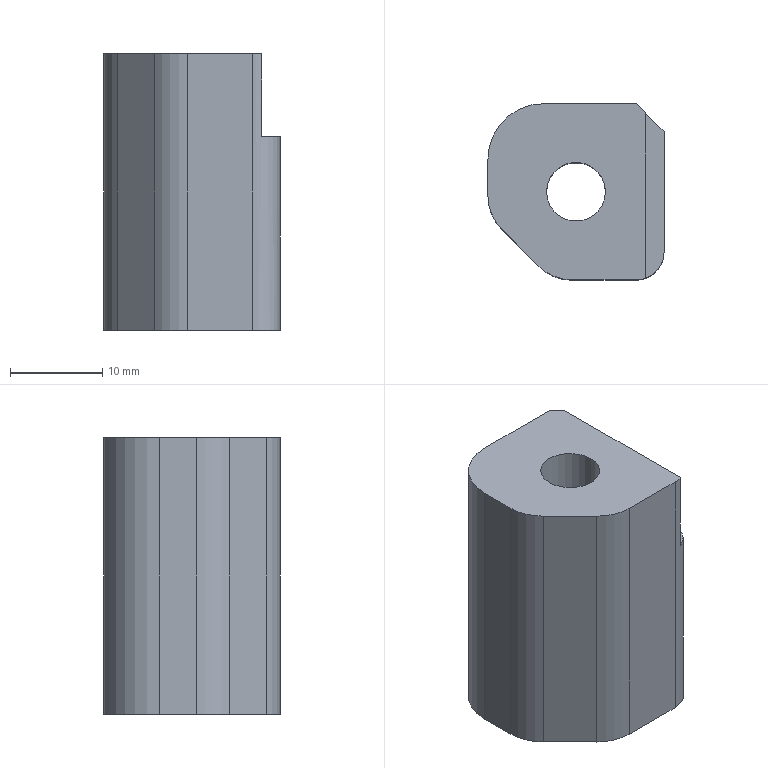Part | STEP file | 1 solid | 15 faces | box 19.1 x 19.1 x 30 mm | volume 8502 mm3 | plane 10 | cylinder 5 | commonest cylinder face diameters 10 x2 6 x1 6.38 x1 12 x1
STEP:
#1=CARTESIAN_POINT('',(-238.45,-56.55,-2.));
#2=VERTEX_POINT('',#1);
#3=CARTESIAN_POINT('',(-245.479,-56.55,-2.));
#4=VERTEX_POINT('',#3);
#5=CARTESIAN_POINT('',(-245.,-56.55,-2.));
#6=DIRECTION('',(-1.,0.,0.));
#7=VECTOR('',#6,1.);
#8=LINE('',#5,#7);
#9=EDGE_CURVE('',#2,#4,#8,.T.);
#10=ORIENTED_EDGE('',*,*,#9,.T.);
#11=CARTESIAN_POINT('',(-245.479,-56.55,-32.));
#12=VERTEX_POINT('',#11);
#13=CARTESIAN_POINT('',(-245.479,-56.55,-30.));
#14=DIRECTION('',(0.,0.,-1.));
#15=VECTOR('',#14,1.);
#16=LINE('',#13,#15);
#17=EDGE_CURVE('',#4,#12,#16,.T.);
#18=ORIENTED_EDGE('',*,*,#17,.T.);
#19=CARTESIAN_POINT('',(-238.45,-56.55,-32.));
#20=VERTEX_POINT('',#19);
#21=CARTESIAN_POINT('',(-245.,-56.55,-32.));
#22=DIRECTION('',(1.,0.,0.));
#23=VECTOR('',#22,1.);
#24=LINE('',#21,#23);
#25=EDGE_CURVE('',#12,#20,#24,.T.);
#26=ORIENTED_EDGE('',*,*,#25,.T.);
#27=CARTESIAN_POINT('',(-238.45,-56.55,-30.));
#28=DIRECTION('',(0.,0.,1.));
#29=VECTOR('',#28,1.);
#30=LINE('',#27,#29);
#31=EDGE_CURVE('',#20,#2,#30,.T.);
#32=ORIENTED_EDGE('',*,*,#31,.T.);
#33=EDGE_LOOP('',(#10,#18,#26,#32));
#34=FACE_OUTER_BOUND('',#33,.T.);
#35=CARTESIAN_POINT('',(-245.,-56.55,-30.));
#36=DIRECTION('',(0.,-1.,0.));
#37=DIRECTION('',(0.,0.,-1.));
#38=AXIS2_PLACEMENT_3D('',#35,#36,#37);
#39=PLANE('',#38);
#40=ADVANCED_FACE('',(#34),#39,.T.);
#41=CARTESIAN_POINT('',(-254.55,-43.45,-32.));
#42=VERTEX_POINT('',#41);
#43=CARTESIAN_POINT('',(-254.55,-47.479,-32.));
#44=VERTEX_POINT('',#43);
#45=CARTESIAN_POINT('',(-254.55,-47.,-32.));
#46=DIRECTION('',(0.,-1.,0.));
#47=VECTOR('',#46,1.);
#48=LINE('',#45,#47);
#49=EDGE_CURVE('',#42,#44,#48,.T.);
#50=ORIENTED_EDGE('',*,*,#49,.T.);
#51=CARTESIAN_POINT('',(-254.55,-47.479,-2.));
#52=VERTEX_POINT('',#51);
#53=CARTESIAN_POINT('',(-254.55,-47.479,-30.));
#54=DIRECTION('',(0.,0.,1.));
#55=VECTOR('',#54,1.);
#56=LINE('',#53,#55);
#57=EDGE_CURVE('',#44,#52,#56,.T.);
#58=ORIENTED_EDGE('',*,*,#57,.T.);
#59=CARTESIAN_POINT('',(-254.55,-43.45,-2.));
#60=VERTEX_POINT('',#59);
#61=CARTESIAN_POINT('',(-254.55,-47.,-2.));
#62=DIRECTION('',(0.,1.,0.));
#63=VECTOR('',#62,1.);
#64=LINE('',#61,#63);
#65=EDGE_CURVE('',#52,#60,#64,.T.);
#66=ORIENTED_EDGE('',*,*,#65,.T.);
#67=CARTESIAN_POINT('',(-254.55,-43.45,-30.));
#68=DIRECTION('',(0.,0.,-1.));
#69=VECTOR('',#68,1.);
#70=LINE('',#67,#69);
#71=EDGE_CURVE('',#60,#42,#70,.T.);
#72=ORIENTED_EDGE('',*,*,#71,.T.);
#73=EDGE_LOOP('',(#50,#58,#66,#72));
#74=FACE_OUTER_BOUND('',#73,.T.);
#75=CARTESIAN_POINT('',(-254.55,-47.,-30.));
#76=DIRECTION('',(-1.,0.,0.));
#77=DIRECTION('',(0.,0.,1.));
#78=AXIS2_PLACEMENT_3D('',#75,#76,#77);
#79=PLANE('',#78);
#80=ADVANCED_FACE('',(#74),#79,.T.);
#81=CARTESIAN_POINT('',(-248.55,-37.45,-32.));
#82=VERTEX_POINT('',#81);
#83=CARTESIAN_POINT('',(-248.55,-37.45,-2.));
#84=VERTEX_POINT('',#83);
#85=CARTESIAN_POINT('',(-248.55,-37.45,-30.));
#86=DIRECTION('',(0.,0.,1.));
#87=VECTOR('',#86,1.);
#88=LINE('',#85,#87);
#89=EDGE_CURVE('',#82,#84,#88,.T.);
#90=ORIENTED_EDGE('',*,*,#89,.T.);
#91=CARTESIAN_POINT('',(-238.45,-37.45,-2.));
#92=VERTEX_POINT('',#91);
#93=CARTESIAN_POINT('',(-245.,-37.45,-2.));
#94=DIRECTION('',(1.,0.,0.));
#95=VECTOR('',#94,1.);
#96=LINE('',#93,#95);
#97=EDGE_CURVE('',#84,#92,#96,.T.);
#98=ORIENTED_EDGE('',*,*,#97,.T.);
#99=CARTESIAN_POINT('',(-238.45,-37.45,-32.));
#100=VERTEX_POINT('',#99);
#101=CARTESIAN_POINT('',(-238.45,-37.45,-30.));
#102=DIRECTION('',(0.,0.,-1.));
#103=VECTOR('',#102,1.);
#104=LINE('',#101,#103);
#105=EDGE_CURVE('',#92,#100,#104,.T.);
#106=ORIENTED_EDGE('',*,*,#105,.T.);
#107=CARTESIAN_POINT('',(-245.,-37.45,-32.));
#108=DIRECTION('',(-1.,0.,0.));
#109=VECTOR('',#108,1.);
#110=LINE('',#107,#109);
#111=EDGE_CURVE('',#100,#82,#110,.T.);
#112=ORIENTED_EDGE('',*,*,#111,.T.);
#113=EDGE_LOOP('',(#90,#98,#106,#112));
#114=FACE_OUTER_BOUND('',#113,.T.);
#115=CARTESIAN_POINT('',(-245.,-37.45,-30.));
#116=DIRECTION('',(0.,1.,0.));
#117=DIRECTION('',(0.,0.,1.));
#118=AXIS2_PLACEMENT_3D('',#115,#116,#117);
#119=PLANE('',#118);
#120=ADVANCED_FACE('',(#114),#119,.T.);
#121=CARTESIAN_POINT('',(-248.19,-47.,-32.));
#122=VERTEX_POINT('',#121);
#123=CARTESIAN_POINT('',(-245.,-47.,-32.));
#124=DIRECTION('',(0.,0.,1.));
#125=DIRECTION('',(-1.,0.,0.));
#126=AXIS2_PLACEMENT_3D('',#123,#124,#125);
#127=CIRCLE('',#126,3.19);
#128=EDGE_CURVE('',#122,#122,#127,.T.);
#129=ORIENTED_EDGE('',*,*,#128,.T.);
#130=EDGE_LOOP('',(#129));
#131=FACE_BOUND('',#130,.T.);
#132=ORIENTED_EDGE('',*,*,#25,.F.);
#133=CARTESIAN_POINT('',(-249.014,-55.086,-32.));
#134=VERTEX_POINT('',#133);
#135=CARTESIAN_POINT('',(-245.479,-51.55,-32.));
#136=DIRECTION('',(0.,0.,-1.));
#137=DIRECTION('',(-1.,0.,0.));
#138=AXIS2_PLACEMENT_3D('',#135,#136,#137);
#139=CIRCLE('',#138,5.);
#140=EDGE_CURVE('',#12,#134,#139,.T.);
#141=ORIENTED_EDGE('',*,*,#140,.T.);
#142=CARTESIAN_POINT('',(-253.086,-51.014,-32.));
#143=VERTEX_POINT('',#142);
#144=CARTESIAN_POINT('',(-251.05,-53.05,-32.));
#145=DIRECTION('',(-0.7071,0.7071,0.));
#146=VECTOR('',#145,1.);
#147=LINE('',#144,#146);
#148=EDGE_CURVE('',#134,#143,#147,.T.);
#149=ORIENTED_EDGE('',*,*,#148,.T.);
#150=CARTESIAN_POINT('',(-249.55,-47.479,-32.));
#151=DIRECTION('',(0.,0.,-1.));
#152=DIRECTION('',(-1.,0.,0.));
#153=AXIS2_PLACEMENT_3D('',#150,#151,#152);
#154=CIRCLE('',#153,5.);
#155=EDGE_CURVE('',#143,#44,#154,.T.);
#156=ORIENTED_EDGE('',*,*,#155,.T.);
#157=ORIENTED_EDGE('',*,*,#49,.F.);
#158=CARTESIAN_POINT('',(-248.55,-43.45,-32.));
#159=DIRECTION('',(0.,0.,-1.));
#160=DIRECTION('',(-1.,0.,0.));
#161=AXIS2_PLACEMENT_3D('',#158,#159,#160);
#162=CIRCLE('',#161,6.);
#163=EDGE_CURVE('',#42,#82,#162,.T.);
#164=ORIENTED_EDGE('',*,*,#163,.T.);
#165=ORIENTED_EDGE('',*,*,#111,.F.);
#166=CARTESIAN_POINT('',(-235.45,-40.45,-32.));
#167=VERTEX_POINT('',#166);
#168=CARTESIAN_POINT('',(-236.95,-38.95,-32.));
#169=DIRECTION('',(0.7071,-0.7071,0.));
#170=VECTOR('',#169,1.);
#171=LINE('',#168,#170);
#172=EDGE_CURVE('',#100,#167,#171,.T.);
#173=ORIENTED_EDGE('',*,*,#172,.T.);
#174=CARTESIAN_POINT('',(-235.45,-53.55,-32.));
#175=VERTEX_POINT('',#174);
#176=CARTESIAN_POINT('',(-235.45,-47.,-32.));
#177=DIRECTION('',(0.,1.,0.));
#178=VECTOR('',#177,1.);
#179=LINE('',#176,#178);
#180=EDGE_CURVE('',#175,#167,#179,.T.);
#181=ORIENTED_EDGE('',*,*,#180,.F.);
#182=CARTESIAN_POINT('',(-238.45,-53.55,-32.));
#183=DIRECTION('',(0.,0.,-1.));
#184=DIRECTION('',(-1.,0.,0.));
#185=AXIS2_PLACEMENT_3D('',#182,#183,#184);
#186=CIRCLE('',#185,3.);
#187=EDGE_CURVE('',#175,#20,#186,.T.);
#188=ORIENTED_EDGE('',*,*,#187,.T.);
#189=EDGE_LOOP('',(#132,#141,#149,#156,#157,#164,#165,#173,#181,#188));
#190=FACE_BOUND('',#189,.T.);
#191=CARTESIAN_POINT('',(-245.,-47.,-32.));
#192=DIRECTION('',(0.,0.,-1.));
#193=DIRECTION('',(-1.,0.,0.));
#194=AXIS2_PLACEMENT_3D('',#191,#192,#193);
#195=PLANE('',#194);
#196=ADVANCED_FACE('',(#131,#190),#195,.T.);
#197=CARTESIAN_POINT('',(-235.45,-40.45,-11.));
#198=VERTEX_POINT('',#197);
#199=CARTESIAN_POINT('',(-235.45,-53.55,-11.));
#200=VERTEX_POINT('',#199);
#201=CARTESIAN_POINT('',(-235.45,-47.,-11.));
#202=DIRECTION('',(0.,-1.,0.));
#203=VECTOR('',#202,1.);
#204=LINE('',#201,#203);
#205=EDGE_CURVE('',#198,#200,#204,.T.);
#206=ORIENTED_EDGE('',*,*,#205,.T.);
#207=CARTESIAN_POINT('',(-235.45,-53.55,-30.));
#208=DIRECTION('',(0.,0.,-1.));
#209=VECTOR('',#208,1.);
#210=LINE('',#207,#209);
#211=EDGE_CURVE('',#200,#175,#210,.T.);
#212=ORIENTED_EDGE('',*,*,#211,.T.);
#213=ORIENTED_EDGE('',*,*,#180,.T.);
#214=CARTESIAN_POINT('',(-235.45,-40.45,-30.));
#215=DIRECTION('',(0.,0.,1.));
#216=VECTOR('',#215,1.);
#217=LINE('',#214,#216);
#218=EDGE_CURVE('',#167,#198,#217,.T.);
#219=ORIENTED_EDGE('',*,*,#218,.T.);
#220=EDGE_LOOP('',(#206,#212,#213,#219));
#221=FACE_OUTER_BOUND('',#220,.T.);
#222=CARTESIAN_POINT('',(-235.45,-47.,-30.));
#223=DIRECTION('',(1.,0.,0.));
#224=DIRECTION('',(0.,0.,-1.));
#225=AXIS2_PLACEMENT_3D('',#222,#223,#224);
#226=PLANE('',#225);
#227=ADVANCED_FACE('',(#221),#226,.T.);
#228=ORIENTED_EDGE('',*,*,#128,.F.);
#229=EDGE_LOOP('',(#228));
#230=FACE_BOUND('',#229,.T.);
#231=CARTESIAN_POINT('',(-241.81,-47.,-2.));
#232=VERTEX_POINT('',#231);
#233=CARTESIAN_POINT('',(-245.,-47.,-2.));
#234=DIRECTION('',(0.,0.,1.));
#235=DIRECTION('',(1.,0.,0.));
#236=AXIS2_PLACEMENT_3D('',#233,#234,#235);
#237=CIRCLE('',#236,3.19);
#238=EDGE_CURVE('',#232,#232,#237,.T.);
#239=ORIENTED_EDGE('',*,*,#238,.T.);
#240=EDGE_LOOP('',(#239));
#241=FACE_BOUND('',#240,.T.);
#242=CARTESIAN_POINT('',(-245.,-47.,-30.));
#243=DIRECTION('',(0.,0.,1.));
#244=DIRECTION('',(1.,0.,0.));
#245=AXIS2_PLACEMENT_3D('',#242,#243,#244);
#246=CYLINDRICAL_SURFACE('',#245,3.19);
#247=ADVANCED_FACE('',(#230,#241),#246,.F.);
#248=ORIENTED_EDGE('',*,*,#71,.F.);
#249=CARTESIAN_POINT('',(-248.55,-43.45,-2.));
#250=DIRECTION('',(0.,0.,1.));
#251=DIRECTION('',(1.,0.,0.));
#252=AXIS2_PLACEMENT_3D('',#249,#250,#251);
#253=CIRCLE('',#252,6.);
#254=EDGE_CURVE('',#84,#60,#253,.T.);
#255=ORIENTED_EDGE('',*,*,#254,.F.);
#256=ORIENTED_EDGE('',*,*,#89,.F.);
#257=ORIENTED_EDGE('',*,*,#163,.F.);
#258=EDGE_LOOP('',(#248,#255,#256,#257));
#259=FACE_OUTER_BOUND('',#258,.T.);
#260=CARTESIAN_POINT('',(-248.55,-43.45,-30.));
#261=DIRECTION('',(0.,0.,1.));
#262=DIRECTION('',(1.,0.,0.));
#263=AXIS2_PLACEMENT_3D('',#260,#261,#262);
#264=CYLINDRICAL_SURFACE('',#263,6.);
#265=ADVANCED_FACE('',(#259),#264,.T.);
#266=ORIENTED_EDGE('',*,*,#105,.F.);
#267=CARTESIAN_POINT('',(-237.45,-38.45,-2.));
#268=VERTEX_POINT('',#267);
#269=CARTESIAN_POINT('',(-236.95,-38.95,-2.));
#270=DIRECTION('',(-0.7071,0.7071,0.));
#271=VECTOR('',#270,1.);
#272=LINE('',#269,#271);
#273=EDGE_CURVE('',#268,#92,#272,.T.);
#274=ORIENTED_EDGE('',*,*,#273,.F.);
#275=CARTESIAN_POINT('',(-237.45,-38.45,-11.));
#276=VERTEX_POINT('',#275);
#277=CARTESIAN_POINT('',(-237.45,-38.45,-30.));
#278=DIRECTION('',(0.,0.,1.));
#279=VECTOR('',#278,1.);
#280=LINE('',#277,#279);
#281=EDGE_CURVE('',#276,#268,#280,.T.);
#282=ORIENTED_EDGE('',*,*,#281,.F.);
#283=CARTESIAN_POINT('',(-236.95,-38.95,-11.));
#284=DIRECTION('',(0.7071,-0.7071,0.));
#285=VECTOR('',#284,1.);
#286=LINE('',#283,#285);
#287=EDGE_CURVE('',#276,#198,#286,.T.);
#288=ORIENTED_EDGE('',*,*,#287,.T.);
#289=ORIENTED_EDGE('',*,*,#218,.F.);
#290=ORIENTED_EDGE('',*,*,#172,.F.);
#291=EDGE_LOOP('',(#266,#274,#282,#288,#289,#290));
#292=FACE_OUTER_BOUND('',#291,.T.);
#293=CARTESIAN_POINT('',(-235.45,-40.45,-30.));
#294=DIRECTION('',(-0.7071,-0.7071,0.));
#295=DIRECTION('',(0.,0.,1.));
#296=AXIS2_PLACEMENT_3D('',#293,#294,#295);
#297=PLANE('',#296);
#298=ADVANCED_FACE('',(#292),#297,.F.);
#299=CARTESIAN_POINT('',(-237.45,-56.378,-11.));
#300=VERTEX_POINT('',#299);
#301=CARTESIAN_POINT('',(-237.45,-45.5,-11.));
#302=DIRECTION('',(0.,-1.,0.));
#303=VECTOR('',#302,1.);
#304=LINE('',#301,#303);
#305=EDGE_CURVE('',#276,#300,#304,.T.);
#306=ORIENTED_EDGE('',*,*,#305,.T.);
#307=CARTESIAN_POINT('',(-238.45,-53.55,-11.));
#308=DIRECTION('',(0.,0.,1.));
#309=DIRECTION('',(-1.,0.,0.));
#310=AXIS2_PLACEMENT_3D('',#307,#308,#309);
#311=CIRCLE('',#310,3.);
#312=EDGE_CURVE('',#300,#200,#311,.T.);
#313=ORIENTED_EDGE('',*,*,#312,.T.);
#314=ORIENTED_EDGE('',*,*,#205,.F.);
#315=ORIENTED_EDGE('',*,*,#287,.F.);
#316=EDGE_LOOP('',(#306,#313,#314,#315));
#317=FACE_OUTER_BOUND('',#316,.T.);
#318=CARTESIAN_POINT('',(-245.,-47.,-11.));
#319=DIRECTION('',(0.,0.,-1.));
#320=DIRECTION('',(-1.,0.,0.));
#321=AXIS2_PLACEMENT_3D('',#318,#319,#320);
#322=PLANE('',#321);
#323=ADVANCED_FACE('',(#317),#322,.F.);
#324=CARTESIAN_POINT('',(-253.086,-51.014,-2.));
#325=VERTEX_POINT('',#324);
#326=CARTESIAN_POINT('',(-249.014,-55.086,-2.));
#327=VERTEX_POINT('',#326);
#328=CARTESIAN_POINT('',(-251.05,-53.05,-2.));
#329=DIRECTION('',(0.7071,-0.7071,0.));
#330=VECTOR('',#329,1.);
#331=LINE('',#328,#330);
#332=EDGE_CURVE('',#325,#327,#331,.T.);
#333=ORIENTED_EDGE('',*,*,#332,.T.);
#334=CARTESIAN_POINT('',(-245.479,-51.55,-2.));
#335=DIRECTION('',(0.,0.,1.));
#336=DIRECTION('',(1.,0.,0.));
#337=AXIS2_PLACEMENT_3D('',#334,#335,#336);
#338=CIRCLE('',#337,5.);
#339=EDGE_CURVE('',#327,#4,#338,.T.);
#340=ORIENTED_EDGE('',*,*,#339,.T.);
#341=ORIENTED_EDGE('',*,*,#9,.F.);
#342=CARTESIAN_POINT('',(-237.45,-56.378,-2.));
#343=VERTEX_POINT('',#342);
#344=CARTESIAN_POINT('',(-238.45,-53.55,-2.));
#345=DIRECTION('',(0.,0.,1.));
#346=DIRECTION('',(1.,0.,0.));
#347=AXIS2_PLACEMENT_3D('',#344,#345,#346);
#348=CIRCLE('',#347,3.);
#349=EDGE_CURVE('',#2,#343,#348,.T.);
#350=ORIENTED_EDGE('',*,*,#349,.T.);
#351=CARTESIAN_POINT('',(-237.45,-45.5,-2.));
#352=DIRECTION('',(0.,1.,0.));
#353=VECTOR('',#352,1.);
#354=LINE('',#351,#353);
#355=EDGE_CURVE('',#343,#268,#354,.T.);
#356=ORIENTED_EDGE('',*,*,#355,.T.);
#357=ORIENTED_EDGE('',*,*,#273,.T.);
#358=ORIENTED_EDGE('',*,*,#97,.F.);
#359=ORIENTED_EDGE('',*,*,#254,.T.);
#360=ORIENTED_EDGE('',*,*,#65,.F.);
#361=CARTESIAN_POINT('',(-249.55,-47.479,-2.));
#362=DIRECTION('',(0.,0.,1.));
#363=DIRECTION('',(1.,0.,0.));
#364=AXIS2_PLACEMENT_3D('',#361,#362,#363);
#365=CIRCLE('',#364,5.);
#366=EDGE_CURVE('',#52,#325,#365,.T.);
#367=ORIENTED_EDGE('',*,*,#366,.T.);
#368=EDGE_LOOP('',(#333,#340,#341,#350,#356,#357,#358,#359,#360,#367));
#369=FACE_BOUND('',#368,.T.);
#370=ORIENTED_EDGE('',*,*,#238,.F.);
#371=EDGE_LOOP('',(#370));
#372=FACE_BOUND('',#371,.T.);
#373=CARTESIAN_POINT('',(-245.,-47.,-2.));
#374=DIRECTION('',(0.,0.,1.));
#375=DIRECTION('',(1.,0.,0.));
#376=AXIS2_PLACEMENT_3D('',#373,#374,#375);
#377=PLANE('',#376);
#378=ADVANCED_FACE('',(#369,#372),#377,.T.);
#379=ORIENTED_EDGE('',*,*,#355,.F.);
#380=CARTESIAN_POINT('',(-237.45,-56.378,0.));
#381=DIRECTION('',(0.,0.,-1.));
#382=VECTOR('',#381,1.);
#383=LINE('',#380,#382);
#384=EDGE_CURVE('',#343,#300,#383,.T.);
#385=ORIENTED_EDGE('',*,*,#384,.T.);
#386=ORIENTED_EDGE('',*,*,#305,.F.);
#387=ORIENTED_EDGE('',*,*,#281,.T.);
#388=EDGE_LOOP('',(#379,#385,#386,#387));
#389=FACE_OUTER_BOUND('',#388,.T.);
#390=CARTESIAN_POINT('',(-237.45,-45.5,-4.5));
#391=DIRECTION('',(-1.,0.,0.));
#392=DIRECTION('',(0.,0.,1.));
#393=AXIS2_PLACEMENT_3D('',#390,#391,#392);
#394=PLANE('',#393);
#395=ADVANCED_FACE('',(#389),#394,.F.);
#396=ORIENTED_EDGE('',*,*,#349,.F.);
#397=ORIENTED_EDGE('',*,*,#31,.F.);
#398=ORIENTED_EDGE('',*,*,#187,.F.);
#399=ORIENTED_EDGE('',*,*,#211,.F.);
#400=ORIENTED_EDGE('',*,*,#312,.F.);
#401=ORIENTED_EDGE('',*,*,#384,.F.);
#402=EDGE_LOOP('',(#396,#397,#398,#399,#400,#401));
#403=FACE_OUTER_BOUND('',#402,.T.);
#404=CARTESIAN_POINT('',(-238.45,-53.55,-30.));
#405=DIRECTION('',(0.,0.,-1.));
#406=DIRECTION('',(-1.,0.,0.));
#407=AXIS2_PLACEMENT_3D('',#404,#405,#406);
#408=CYLINDRICAL_SURFACE('',#407,3.);
#409=ADVANCED_FACE('',(#403),#408,.T.);
#410=ORIENTED_EDGE('',*,*,#148,.F.);
#411=CARTESIAN_POINT('',(-249.014,-55.086,-30.));
#412=DIRECTION('',(0.,0.,1.));
#413=VECTOR('',#412,1.);
#414=LINE('',#411,#413);
#415=EDGE_CURVE('',#134,#327,#414,.T.);
#416=ORIENTED_EDGE('',*,*,#415,.T.);
#417=ORIENTED_EDGE('',*,*,#332,.F.);
#418=CARTESIAN_POINT('',(-253.086,-51.014,-30.));
#419=DIRECTION('',(0.,0.,-1.));
#420=VECTOR('',#419,1.);
#421=LINE('',#418,#420);
#422=EDGE_CURVE('',#325,#143,#421,.T.);
#423=ORIENTED_EDGE('',*,*,#422,.T.);
#424=EDGE_LOOP('',(#410,#416,#417,#423));
#425=FACE_OUTER_BOUND('',#424,.T.);
#426=CARTESIAN_POINT('',(-254.55,-49.55,-30.));
#427=DIRECTION('',(0.7071,0.7071,0.));
#428=DIRECTION('',(0.,0.,1.));
#429=AXIS2_PLACEMENT_3D('',#426,#427,#428);
#430=PLANE('',#429);
#431=ADVANCED_FACE('',(#425),#430,.F.);
#432=ORIENTED_EDGE('',*,*,#339,.F.);
#433=ORIENTED_EDGE('',*,*,#415,.F.);
#434=ORIENTED_EDGE('',*,*,#140,.F.);
#435=ORIENTED_EDGE('',*,*,#17,.F.);
#436=EDGE_LOOP('',(#432,#433,#434,#435));
#437=FACE_OUTER_BOUND('',#436,.T.);
#438=CARTESIAN_POINT('',(-245.479,-51.55,-30.));
#439=DIRECTION('',(0.,0.,1.));
#440=DIRECTION('',(1.,0.,0.));
#441=AXIS2_PLACEMENT_3D('',#438,#439,#440);
#442=CYLINDRICAL_SURFACE('',#441,5.);
#443=ADVANCED_FACE('',(#437),#442,.T.);
#444=ORIENTED_EDGE('',*,*,#155,.F.);
#445=ORIENTED_EDGE('',*,*,#422,.F.);
#446=ORIENTED_EDGE('',*,*,#366,.F.);
#447=ORIENTED_EDGE('',*,*,#57,.F.);
#448=EDGE_LOOP('',(#444,#445,#446,#447));
#449=FACE_OUTER_BOUND('',#448,.T.);
#450=CARTESIAN_POINT('',(-249.55,-47.479,-30.));
#451=DIRECTION('',(0.,0.,-1.));
#452=DIRECTION('',(-1.,0.,0.));
#453=AXIS2_PLACEMENT_3D('',#450,#451,#452);
#454=CYLINDRICAL_SURFACE('',#453,5.);
#455=ADVANCED_FACE('',(#449),#454,.T.);
#456=CLOSED_SHELL('',(#40,#80,#120,#196,#227,#247,#265,#298,#323,#378,#395,#409,#431,#443,#455));
#457=MANIFOLD_SOLID_BREP('',#456);
#458=(LENGTH_UNIT()NAMED_UNIT(*)SI_UNIT(.MILLI.,.METRE.));
#459=UNCERTAINTY_MEASURE_WITH_UNIT(LENGTH_MEASURE(0.00002),#458,'','');
#460=(NAMED_UNIT(*)PLANE_ANGLE_UNIT()SI_UNIT($,.RADIAN.));
#461=PLANE_ANGLE_MEASURE_WITH_UNIT(PLANE_ANGLE_MEASURE(0.01745),#460);
#462=DIMENSIONAL_EXPONENTS(0.,0.,0.,0.,0.,0.,0.);
#463=(CONVERSION_BASED_UNIT('DEGREE',#461)NAMED_UNIT(#462)PLANE_ANGLE_UNIT());
#464=(NAMED_UNIT(*)SI_UNIT($,.STERADIAN.)SOLID_ANGLE_UNIT());
#465=(GEOMETRIC_REPRESENTATION_CONTEXT(3)GLOBAL_UNCERTAINTY_ASSIGNED_CONTEXT((#459))GLOBAL_UNIT_ASSIGNED_CONTEXT((#458,#463,#464))REPRESENTATION_CONTEXT('',''));
#466=ADVANCED_BREP_SHAPE_REPRESENTATION('',(#457),#465);